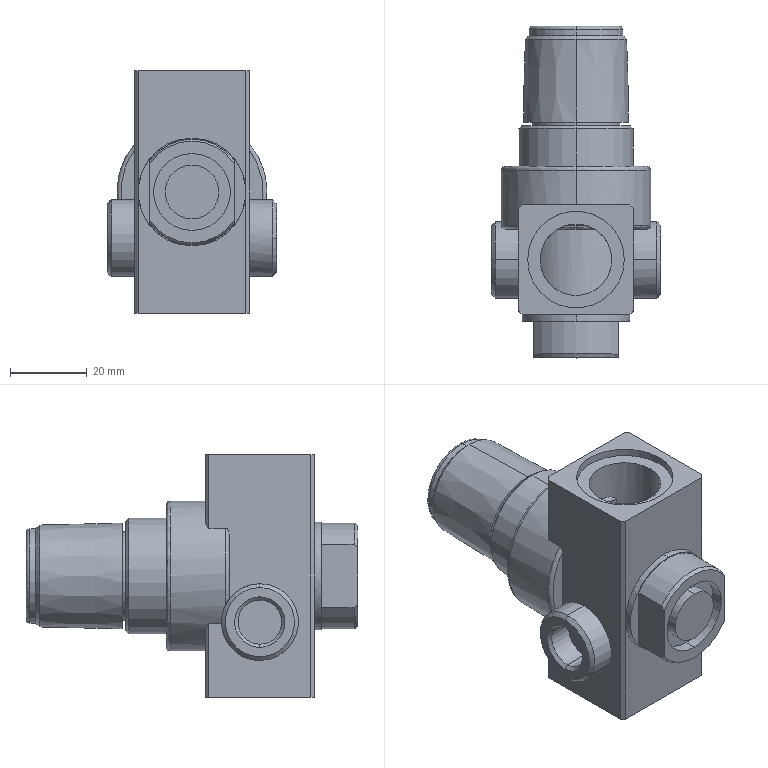Part | STEP file | HI_BR4000 By-BR | 1 solid | 103 faces | box 44 x 86.3 x 63 mm | volume 87528 mm3 | cylinder 44 | plane 34 | cone 16 | spline 9 | commonest cylinder face diameters 18.631 x7 20 x7 11.445 x5 28 x5 39 x5 25.146 x4